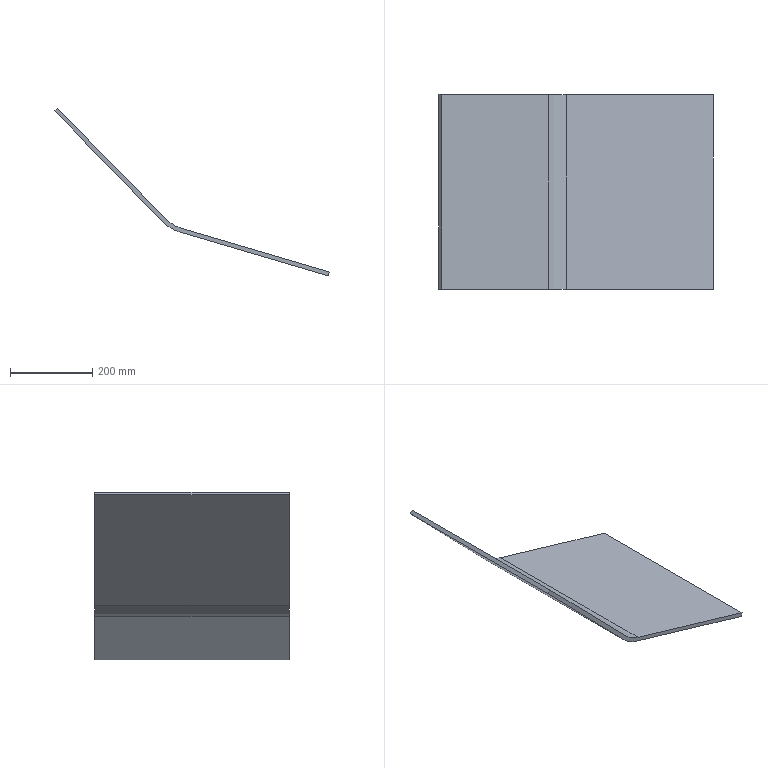Part | SolidWorks | features Extrusion 1, Fillet 1 | 1 solid | 10 faces | box 669.894 x 475 x 409.47 mm | volume 3812408 mm3 | plane 8 | cylinder 2 | commonest cylinder face diameters 200 x2
STEP:
#1=CARTESIAN_POINT('',(-7.163,0.,-6.978));
#2=VERTEX_POINT('',#1);
#3=CARTESIAN_POINT('',(0.,0.,0.));
#4=VERTEX_POINT('',#3);
#5=CARTESIAN_POINT('',(-7.163,0.,-6.978));
#6=DIRECTION('',(0.7163,0.,0.6978));
#7=VECTOR('',#6,1000.);
#8=LINE('',#5,#7);
#9=EDGE_CURVE('',#2,#4,#8,.T.);
#10=ORIENTED_EDGE('',*,*,#9,.T.);
#11=CARTESIAN_POINT('',(0.,475.,0.));
#12=VERTEX_POINT('',#11);
#13=CARTESIAN_POINT('',(0.,475.,0.));
#14=DIRECTION('',(0.,-1.,0.));
#15=VECTOR('',#14,1000.);
#16=LINE('',#13,#15);
#17=EDGE_CURVE('',#12,#4,#16,.T.);
#18=ORIENTED_EDGE('',*,*,#17,.F.);
#19=CARTESIAN_POINT('',(-7.163,475.,-6.978));
#20=VERTEX_POINT('',#19);
#21=CARTESIAN_POINT('',(-7.163,475.,-6.978));
#22=DIRECTION('',(0.7163,0.,0.6978));
#23=VECTOR('',#22,1000.);
#24=LINE('',#21,#23);
#25=EDGE_CURVE('',#20,#12,#24,.T.);
#26=ORIENTED_EDGE('',*,*,#25,.F.);
#27=CARTESIAN_POINT('',(-7.163,475.,-6.978));
#28=DIRECTION('',(0.,-1.,0.));
#29=VECTOR('',#28,1000.);
#30=LINE('',#27,#29);
#31=EDGE_CURVE('',#20,#2,#30,.T.);
#32=ORIENTED_EDGE('',*,*,#31,.T.);
#33=EDGE_LOOP('',(#10,#18,#26,#32));
#34=FACE_OUTER_BOUND('',#33,.T.);
#35=CARTESIAN_POINT('',(-7.163,475.,-6.978));
#36=DIRECTION('',(0.6978,0.,-0.7163));
#37=DIRECTION('',(-0.7163,0.,-0.6978));
#38=AXIS2_PLACEMENT_3D('',#35,#36,#37);
#39=PLANE('',#38);
#40=ADVANCED_FACE('',(#34),#39,.F.);
#41=CARTESIAN_POINT('',(260.907,0.,-267.791));
#42=VERTEX_POINT('',#41);
#43=CARTESIAN_POINT('',(0.,0.,0.));
#44=DIRECTION('',(0.6978,0.,-0.7163));
#45=VECTOR('',#44,1000.);
#46=LINE('',#43,#45);
#47=EDGE_CURVE('',#4,#42,#46,.T.);
#48=ORIENTED_EDGE('',*,*,#47,.T.);
#49=CARTESIAN_POINT('',(260.907,475.,-267.791));
#50=VERTEX_POINT('',#49);
#51=CARTESIAN_POINT('',(260.907,475.,-267.791));
#52=DIRECTION('',(0.,1.,0.));
#53=VECTOR('',#52,1000.);
#54=LINE('',#51,#53);
#55=EDGE_CURVE('',#42,#50,#54,.T.);
#56=ORIENTED_EDGE('',*,*,#55,.T.);
#57=CARTESIAN_POINT('',(0.,475.,0.));
#58=DIRECTION('',(0.6978,0.,-0.7163));
#59=VECTOR('',#58,1000.);
#60=LINE('',#57,#59);
#61=EDGE_CURVE('',#12,#50,#60,.T.);
#62=ORIENTED_EDGE('',*,*,#61,.F.);
#63=ORIENTED_EDGE('',*,*,#17,.T.);
#64=EDGE_LOOP('',(#48,#56,#62,#63));
#65=FACE_OUTER_BOUND('',#64,.T.);
#66=CARTESIAN_POINT('',(0.,475.,0.));
#67=DIRECTION('',(-0.7163,0.,-0.6978));
#68=DIRECTION('',(-0.6978,0.,0.7163));
#69=AXIS2_PLACEMENT_3D('',#66,#67,#68);
#70=PLANE('',#69);
#71=ADVANCED_FACE('',(#65),#70,.F.);
#72=CARTESIAN_POINT('',(304.187,475.,-293.906));
#73=VERTEX_POINT('',#72);
#74=CARTESIAN_POINT('',(662.731,475.,-399.88));
#75=VERTEX_POINT('',#74);
#76=CARTESIAN_POINT('',(279.136,475.,-286.501));
#77=DIRECTION('',(0.959,0.,-0.2834));
#78=VECTOR('',#77,1000.);
#79=LINE('',#76,#78);
#80=EDGE_CURVE('',#73,#75,#79,.T.);
#81=ORIENTED_EDGE('',*,*,#80,.F.);
#82=CARTESIAN_POINT('',(304.187,0.,-293.906));
#83=VERTEX_POINT('',#82);
#84=CARTESIAN_POINT('',(304.187,0.,-293.906));
#85=DIRECTION('',(0.,-1.,0.));
#86=VECTOR('',#85,1000.);
#87=LINE('',#84,#86);
#88=EDGE_CURVE('',#73,#83,#87,.T.);
#89=ORIENTED_EDGE('',*,*,#88,.T.);
#90=CARTESIAN_POINT('',(662.731,0.,-399.88));
#91=VERTEX_POINT('',#90);
#92=CARTESIAN_POINT('',(279.136,0.,-286.501));
#93=DIRECTION('',(0.959,0.,-0.2834));
#94=VECTOR('',#93,1000.);
#95=LINE('',#92,#94);
#96=EDGE_CURVE('',#83,#91,#95,.T.);
#97=ORIENTED_EDGE('',*,*,#96,.T.);
#98=CARTESIAN_POINT('',(662.731,475.,-399.88));
#99=DIRECTION('',(0.,-1.,0.));
#100=VECTOR('',#99,1000.);
#101=LINE('',#98,#100);
#102=EDGE_CURVE('',#75,#91,#101,.T.);
#103=ORIENTED_EDGE('',*,*,#102,.F.);
#104=EDGE_LOOP('',(#81,#89,#97,#103));
#105=FACE_OUTER_BOUND('',#104,.T.);
#106=CARTESIAN_POINT('',(279.136,475.,-286.501));
#107=DIRECTION('',(-0.2834,0.,-0.959));
#108=DIRECTION('',(-0.959,0.,0.2834));
#109=AXIS2_PLACEMENT_3D('',#106,#107,#108);
#110=PLANE('',#109);
#111=ADVANCED_FACE('',(#105),#110,.F.);
#112=CARTESIAN_POINT('',(659.897,0.,-409.47));
#113=VERTEX_POINT('',#112);
#114=CARTESIAN_POINT('',(659.897,0.,-409.47));
#115=DIRECTION('',(-0.2834,0.,-0.959));
#116=VECTOR('',#115,1000.);
#117=LINE('',#114,#116);
#118=EDGE_CURVE('',#91,#113,#117,.T.);
#119=ORIENTED_EDGE('',*,*,#118,.T.);
#120=CARTESIAN_POINT('',(659.897,475.,-409.47));
#121=VERTEX_POINT('',#120);
#122=CARTESIAN_POINT('',(659.897,475.,-409.47));
#123=DIRECTION('',(0.,-1.,0.));
#124=VECTOR('',#123,1000.);
#125=LINE('',#122,#124);
#126=EDGE_CURVE('',#121,#113,#125,.T.);
#127=ORIENTED_EDGE('',*,*,#126,.F.);
#128=CARTESIAN_POINT('',(659.897,475.,-409.47));
#129=DIRECTION('',(-0.2834,0.,-0.959));
#130=VECTOR('',#129,1000.);
#131=LINE('',#128,#130);
#132=EDGE_CURVE('',#75,#121,#131,.T.);
#133=ORIENTED_EDGE('',*,*,#132,.F.);
#134=ORIENTED_EDGE('',*,*,#102,.T.);
#135=EDGE_LOOP('',(#119,#127,#133,#134));
#136=FACE_OUTER_BOUND('',#135,.T.);
#137=CARTESIAN_POINT('',(659.897,475.,-409.47));
#138=DIRECTION('',(-0.959,0.,0.2834));
#139=DIRECTION('',(0.2834,0.,0.959));
#140=AXIS2_PLACEMENT_3D('',#137,#138,#139);
#141=PLANE('',#140);
#142=ADVANCED_FACE('',(#136),#141,.F.);
#143=CARTESIAN_POINT('',(298.848,0.,-302.755));
#144=VERTEX_POINT('',#143);
#145=CARTESIAN_POINT('',(273.797,0.,-295.351));
#146=DIRECTION('',(-0.959,0.,0.2834));
#147=VECTOR('',#146,1000.);
#148=LINE('',#145,#147);
#149=EDGE_CURVE('',#113,#144,#148,.T.);
#150=ORIENTED_EDGE('',*,*,#149,.T.);
#151=CARTESIAN_POINT('',(298.848,475.,-302.755));
#152=VERTEX_POINT('',#151);
#153=CARTESIAN_POINT('',(298.848,475.,-302.755));
#154=DIRECTION('',(0.,1.,0.));
#155=VECTOR('',#154,1000.);
#156=LINE('',#153,#155);
#157=EDGE_CURVE('',#144,#152,#156,.T.);
#158=ORIENTED_EDGE('',*,*,#157,.T.);
#159=CARTESIAN_POINT('',(273.797,475.,-295.351));
#160=DIRECTION('',(-0.959,0.,0.2834));
#161=VECTOR('',#160,1000.);
#162=LINE('',#159,#161);
#163=EDGE_CURVE('',#121,#152,#162,.T.);
#164=ORIENTED_EDGE('',*,*,#163,.F.);
#165=ORIENTED_EDGE('',*,*,#126,.T.);
#166=EDGE_LOOP('',(#150,#158,#164,#165));
#167=FACE_OUTER_BOUND('',#166,.T.);
#168=CARTESIAN_POINT('',(273.797,475.,-295.351));
#169=DIRECTION('',(0.2834,0.,0.959));
#170=DIRECTION('',(0.959,0.,-0.2834));
#171=AXIS2_PLACEMENT_3D('',#168,#169,#170);
#172=PLANE('',#171);
#173=ADVANCED_FACE('',(#167),#172,.F.);
#174=CARTESIAN_POINT('',(255.567,475.,-276.64));
#175=VERTEX_POINT('',#174);
#176=CARTESIAN_POINT('',(-7.163,475.,-6.978));
#177=DIRECTION('',(-0.6978,0.,0.7163));
#178=VECTOR('',#177,1000.);
#179=LINE('',#176,#178);
#180=EDGE_CURVE('',#175,#20,#179,.T.);
#181=ORIENTED_EDGE('',*,*,#180,.F.);
#182=CARTESIAN_POINT('',(255.567,0.,-276.64));
#183=VERTEX_POINT('',#182);
#184=CARTESIAN_POINT('',(255.567,475.,-276.64));
#185=DIRECTION('',(0.,-1.,0.));
#186=VECTOR('',#185,1000.);
#187=LINE('',#184,#186);
#188=EDGE_CURVE('',#175,#183,#187,.T.);
#189=ORIENTED_EDGE('',*,*,#188,.T.);
#190=CARTESIAN_POINT('',(-7.163,0.,-6.978));
#191=DIRECTION('',(-0.6978,0.,0.7163));
#192=VECTOR('',#191,1000.);
#193=LINE('',#190,#192);
#194=EDGE_CURVE('',#183,#2,#193,.T.);
#195=ORIENTED_EDGE('',*,*,#194,.T.);
#196=ORIENTED_EDGE('',*,*,#31,.F.);
#197=EDGE_LOOP('',(#181,#189,#195,#196));
#198=FACE_OUTER_BOUND('',#197,.T.);
#199=CARTESIAN_POINT('',(-7.163,475.,-6.978));
#200=DIRECTION('',(0.7163,0.,0.6978));
#201=DIRECTION('',(0.6978,0.,-0.7163));
#202=AXIS2_PLACEMENT_3D('',#199,#200,#201);
#203=PLANE('',#202);
#204=ADVANCED_FACE('',(#198),#203,.F.);
#205=ORIENTED_EDGE('',*,*,#163,.T.);
#206=CARTESIAN_POINT('',(327.193,475.,-206.856));
#207=DIRECTION('',(0.,1.,0.));
#208=DIRECTION('',(0.,0.,1.));
#209=AXIS2_PLACEMENT_3D('',#206,#207,#208);
#210=CIRCLE('',#209,100.);
#211=EDGE_CURVE('',#152,#175,#210,.T.);
#212=ORIENTED_EDGE('',*,*,#211,.T.);
#213=ORIENTED_EDGE('',*,*,#180,.T.);
#214=ORIENTED_EDGE('',*,*,#25,.T.);
#215=ORIENTED_EDGE('',*,*,#61,.T.);
#216=CARTESIAN_POINT('',(332.532,475.,-198.007));
#217=DIRECTION('',(0.,-1.,0.));
#218=DIRECTION('',(0.,0.,1.));
#219=AXIS2_PLACEMENT_3D('',#216,#217,#218);
#220=CIRCLE('',#219,100.);
#221=EDGE_CURVE('',#50,#73,#220,.T.);
#222=ORIENTED_EDGE('',*,*,#221,.T.);
#223=ORIENTED_EDGE('',*,*,#80,.T.);
#224=ORIENTED_EDGE('',*,*,#132,.T.);
#225=EDGE_LOOP('',(#205,#212,#213,#214,#215,#222,#223,#224));
#226=FACE_OUTER_BOUND('',#225,.T.);
#227=CARTESIAN_POINT('',(0.,475.,0.));
#228=DIRECTION('',(0.,1.,0.));
#229=DIRECTION('',(0.,0.,1.));
#230=AXIS2_PLACEMENT_3D('',#227,#228,#229);
#231=PLANE('',#230);
#232=ADVANCED_FACE('',(#226),#231,.T.);
#233=ORIENTED_EDGE('',*,*,#194,.F.);
#234=CARTESIAN_POINT('',(327.193,0.,-206.856));
#235=DIRECTION('',(0.,-1.,0.));
#236=DIRECTION('',(0.,0.,1.));
#237=AXIS2_PLACEMENT_3D('',#234,#235,#236);
#238=CIRCLE('',#237,100.);
#239=EDGE_CURVE('',#183,#144,#238,.T.);
#240=ORIENTED_EDGE('',*,*,#239,.T.);
#241=ORIENTED_EDGE('',*,*,#149,.F.);
#242=ORIENTED_EDGE('',*,*,#118,.F.);
#243=ORIENTED_EDGE('',*,*,#96,.F.);
#244=CARTESIAN_POINT('',(332.532,0.,-198.007));
#245=DIRECTION('',(0.,1.,0.));
#246=DIRECTION('',(0.,0.,1.));
#247=AXIS2_PLACEMENT_3D('',#244,#245,#246);
#248=CIRCLE('',#247,100.);
#249=EDGE_CURVE('',#83,#42,#248,.T.);
#250=ORIENTED_EDGE('',*,*,#249,.T.);
#251=ORIENTED_EDGE('',*,*,#47,.F.);
#252=ORIENTED_EDGE('',*,*,#9,.F.);
#253=EDGE_LOOP('',(#233,#240,#241,#242,#243,#250,#251,#252));
#254=FACE_OUTER_BOUND('',#253,.T.);
#255=CARTESIAN_POINT('',(0.,0.,0.));
#256=DIRECTION('',(0.,1.,0.));
#257=DIRECTION('',(0.,0.,1.));
#258=AXIS2_PLACEMENT_3D('',#255,#256,#257);
#259=PLANE('',#258);
#260=ADVANCED_FACE('',(#254),#259,.F.);
#261=ORIENTED_EDGE('',*,*,#221,.F.);
#262=ORIENTED_EDGE('',*,*,#55,.F.);
#263=ORIENTED_EDGE('',*,*,#249,.F.);
#264=ORIENTED_EDGE('',*,*,#88,.F.);
#265=EDGE_LOOP('',(#261,#262,#263,#264));
#266=FACE_OUTER_BOUND('',#265,.T.);
#267=CARTESIAN_POINT('',(332.532,475.,-198.007));
#268=DIRECTION('',(0.,1.,0.));
#269=DIRECTION('',(0.,0.,1.));
#270=AXIS2_PLACEMENT_3D('',#267,#268,#269);
#271=CYLINDRICAL_SURFACE('',#270,100.);
#272=ADVANCED_FACE('',(#266),#271,.F.);
#273=ORIENTED_EDGE('',*,*,#211,.F.);
#274=ORIENTED_EDGE('',*,*,#157,.F.);
#275=ORIENTED_EDGE('',*,*,#239,.F.);
#276=ORIENTED_EDGE('',*,*,#188,.F.);
#277=EDGE_LOOP('',(#273,#274,#275,#276));
#278=FACE_OUTER_BOUND('',#277,.T.);
#279=CARTESIAN_POINT('',(327.193,475.,-206.856));
#280=DIRECTION('',(0.,-1.,0.));
#281=DIRECTION('',(0.,0.,-1.));
#282=AXIS2_PLACEMENT_3D('',#279,#280,#281);
#283=CYLINDRICAL_SURFACE('',#282,100.);
#284=ADVANCED_FACE('',(#278),#283,.T.);
#285=CLOSED_SHELL('',(#40,#71,#111,#142,#173,#204,#232,#260,#272,#284));
#286=MANIFOLD_SOLID_BREP('',#285);
#287=CARTESIAN_POINT('',(0.,0.,0.));
#288=DIRECTION('',(0.,0.,1.));
#289=DIRECTION('',(1.,0.,0.));
#290=AXIS2_PLACEMENT_3D('',#287,#288,#289);
#291=(LENGTH_UNIT()NAMED_UNIT(*)SI_UNIT(.MILLI.,.METRE.));
#292=UNCERTAINTY_MEASURE_WITH_UNIT(LENGTH_MEASURE(0.00001),#291,'','');
#293=(NAMED_UNIT(*)PLANE_ANGLE_UNIT()SI_UNIT($,.RADIAN.));
#294=(NAMED_UNIT(*)SI_UNIT($,.STERADIAN.)SOLID_ANGLE_UNIT());
#295=(GEOMETRIC_REPRESENTATION_CONTEXT(3)GLOBAL_UNCERTAINTY_ASSIGNED_CONTEXT((#292))GLOBAL_UNIT_ASSIGNED_CONTEXT((#291,#293,#294))REPRESENTATION_CONTEXT('',''));
#296=ADVANCED_BREP_SHAPE_REPRESENTATION('',(#286,#290),#295);